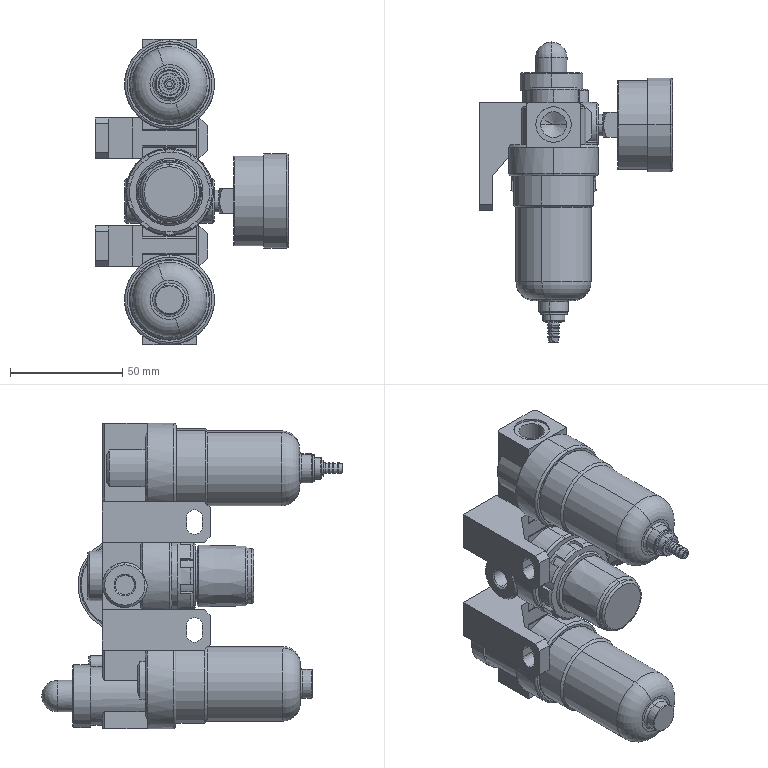Part | STEP file | AC20001 | 11 solids | 504 faces | box 86 x 133.8 x 136 mm | volume 222046 mm3 | plane 228 | cylinder 160 | cone 84 | torus 24 | spline 6 | sphere 2 | commonest cylinder face diameters 11.445 x12 8 x10 35.2 x10 5 x8 6 x8 13 x8